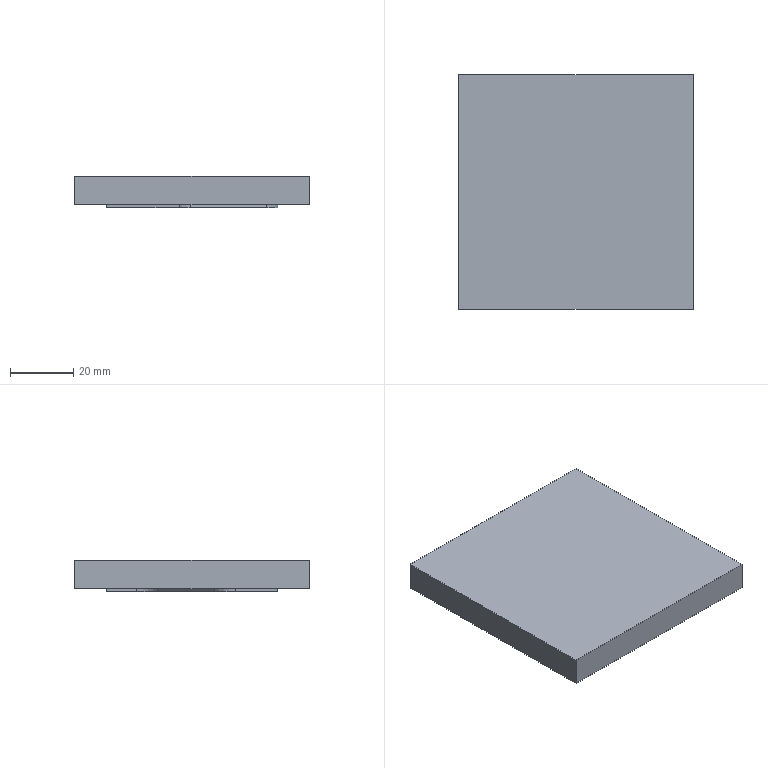NC program | NX | posted with a generic post | part box 74 x 74 x 10 mm
Whole program:
N10 G17 G21 G94 G90
(ZLEVEL_PROFILE_COPY , TOOL : D10JING)
N12 T14 M6
N14 G54
N16 G17 G0 G90 X-19.81 Y6.285 B0. C0. S7500 M3
N18 G43 Z30. H14
N20 Z-3.
N22 G94 G1 Z-4. F1000.
N24 X-21.143 Y5.32
N26 G3 X-20.721 Y4.414 R1.
N28 G1 X3.456 Y-12.516
N30 G2 X8.948 Y-22. R13.
N32 G1 X22.
N34 Y-13.665
N36 G3 X20.721 Y-11.207 R3.
N38 G1 X-4.956 Y6.772
N40 G2 X-10.5 Y17.421 R13.
N42 G1 Y22.
N44 X-22.
N46 Y6.871
N48 G3 X-20.721 Y4.414 R3.
N50 X-19.725 Y4.326 R1.
N52 G1 X-18.155 Y5.058
N54 Z-3.
N56 G0 Z30.
N58 M5
(PLANAR_MILL_COPY_COPY , TOOL : D6A45)
N60 T01 M6
N62 G54
N64 G17 G0 G90 X-11.502 Y-5.582 B0. C0. S7500 M3
N66 G43 Z30. H1
N68 Z1.
N70 G94 G1 Z-1. F1250.
N72 X-11.406 Y-6.678
N74 G3 X-10.984 Y-7.41 R1.
N76 G1 X1.105 Y-15.874
N78 G2 X4.9 Y-23.165 R8.9
N80 G1 Y-26.1
N82 X26.1
N84 Y-13.665
N86 G3 X23.072 Y-7.849 R7.1
N88 G1 X-2.605 Y10.131
N90 G2 X-6.4 Y17.421 R8.9
N92 G1 Y26.1
N94 X-26.1
N96 Y6.871
N98 G3 X-23.072 Y1.055 R7.1
N100 G1 X-10.984 Y-7.41
N102 G3 X-10.151 Y-7.556 R1.
N104 G1 X-9.089 Y-7.272
N106 Z1.
N108 G0 Z30.
N110 M5
N112 M2